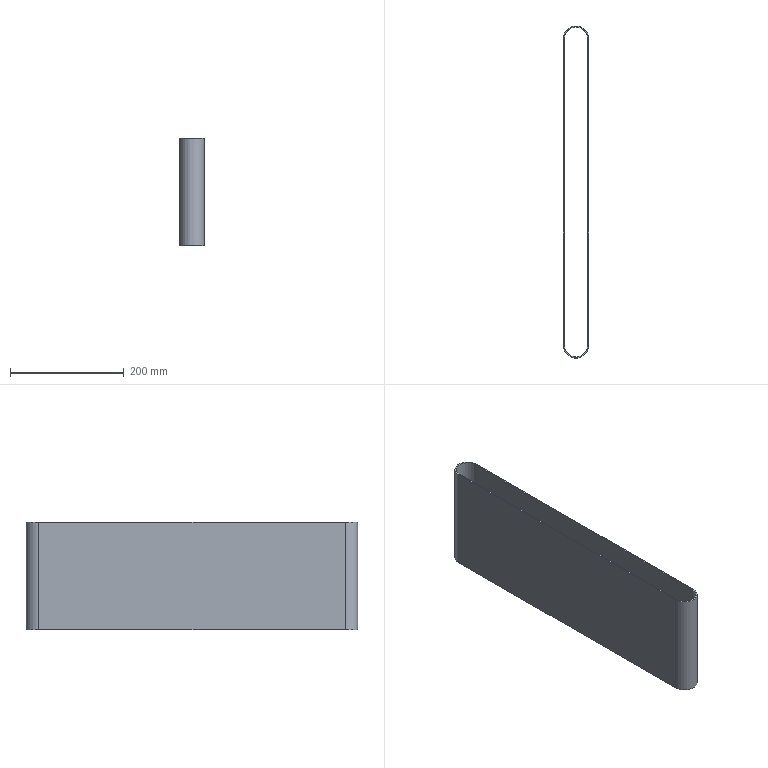Part | SolidWorks | features BeltProfileFeature 1, ExtruThin 1 | 1 solid | 10 faces | box 44.5 x 584.5 x 190 mm | volume 461137 mm3 | plane 6 | cylinder 4 | commonest cylinder face diameters 40.5 x2 44.5 x2
STEP:
#1=CARTESIAN_POINT('',(-22.25,0.,95.));
#2=VERTEX_POINT('',#1);
#3=CARTESIAN_POINT('',(22.25,0.,95.));
#4=VERTEX_POINT('',#3);
#5=CARTESIAN_POINT('',(0.,0.,95.));
#6=DIRECTION('',(0.,0.,1.));
#7=DIRECTION('',(-1.,0.,0.));
#8=AXIS2_PLACEMENT_3D('',#5,#6,#7);
#9=CIRCLE('',#8,22.25);
#10=EDGE_CURVE('',#2,#4,#9,.T.);
#11=ORIENTED_EDGE('',*,*,#10,.T.);
#12=CARTESIAN_POINT('',(22.25,540.,95.));
#13=VERTEX_POINT('',#12);
#14=CARTESIAN_POINT('',(22.25,0.,95.));
#15=DIRECTION('',(0.,1.,0.));
#16=VECTOR('',#15,1000.);
#17=LINE('',#14,#16);
#18=EDGE_CURVE('',#4,#13,#17,.T.);
#19=ORIENTED_EDGE('',*,*,#18,.T.);
#20=CARTESIAN_POINT('',(-22.25,540.,95.));
#21=VERTEX_POINT('',#20);
#22=CARTESIAN_POINT('',(0.,540.,95.));
#23=DIRECTION('',(0.,0.,1.));
#24=DIRECTION('',(-1.,0.,0.));
#25=AXIS2_PLACEMENT_3D('',#22,#23,#24);
#26=CIRCLE('',#25,22.25);
#27=EDGE_CURVE('',#13,#21,#26,.T.);
#28=ORIENTED_EDGE('',*,*,#27,.T.);
#29=CARTESIAN_POINT('',(-22.25,0.,95.));
#30=DIRECTION('',(0.,-1.,0.));
#31=VECTOR('',#30,1000.);
#32=LINE('',#29,#31);
#33=EDGE_CURVE('',#21,#2,#32,.T.);
#34=ORIENTED_EDGE('',*,*,#33,.T.);
#35=EDGE_LOOP('',(#11,#19,#28,#34));
#36=FACE_OUTER_BOUND('',#35,.T.);
#37=CARTESIAN_POINT('',(-20.25,0.,95.));
#38=VERTEX_POINT('',#37);
#39=CARTESIAN_POINT('',(20.25,0.,95.));
#40=VERTEX_POINT('',#39);
#41=CARTESIAN_POINT('',(0.,0.,95.));
#42=DIRECTION('',(0.,0.,1.));
#43=DIRECTION('',(-1.,0.,0.));
#44=AXIS2_PLACEMENT_3D('',#41,#42,#43);
#45=CIRCLE('',#44,20.25);
#46=EDGE_CURVE('',#38,#40,#45,.T.);
#47=ORIENTED_EDGE('',*,*,#46,.F.);
#48=CARTESIAN_POINT('',(-20.25,540.,95.));
#49=VERTEX_POINT('',#48);
#50=CARTESIAN_POINT('',(-20.25,0.,95.));
#51=DIRECTION('',(0.,-1.,0.));
#52=VECTOR('',#51,1000.);
#53=LINE('',#50,#52);
#54=EDGE_CURVE('',#49,#38,#53,.T.);
#55=ORIENTED_EDGE('',*,*,#54,.F.);
#56=CARTESIAN_POINT('',(20.25,540.,95.));
#57=VERTEX_POINT('',#56);
#58=CARTESIAN_POINT('',(0.,540.,95.));
#59=DIRECTION('',(0.,0.,1.));
#60=DIRECTION('',(-1.,0.,0.));
#61=AXIS2_PLACEMENT_3D('',#58,#59,#60);
#62=CIRCLE('',#61,20.25);
#63=EDGE_CURVE('',#57,#49,#62,.T.);
#64=ORIENTED_EDGE('',*,*,#63,.F.);
#65=CARTESIAN_POINT('',(20.25,540.,95.));
#66=DIRECTION('',(0.,1.,0.));
#67=VECTOR('',#66,1000.);
#68=LINE('',#65,#67);
#69=EDGE_CURVE('',#40,#57,#68,.T.);
#70=ORIENTED_EDGE('',*,*,#69,.F.);
#71=EDGE_LOOP('',(#47,#55,#64,#70));
#72=FACE_BOUND('',#71,.T.);
#73=CARTESIAN_POINT('',(0.,0.,95.));
#74=DIRECTION('',(0.,0.,-1.));
#75=DIRECTION('',(-1.,0.,0.));
#76=AXIS2_PLACEMENT_3D('',#73,#74,#75);
#77=PLANE('',#76);
#78=ADVANCED_FACE('',(#36,#72),#77,.F.);
#79=CARTESIAN_POINT('',(-22.25,0.,-95.));
#80=VERTEX_POINT('',#79);
#81=CARTESIAN_POINT('',(22.25,0.,-95.));
#82=VERTEX_POINT('',#81);
#83=CARTESIAN_POINT('',(0.,0.,-95.));
#84=DIRECTION('',(0.,0.,1.));
#85=DIRECTION('',(-1.,0.,0.));
#86=AXIS2_PLACEMENT_3D('',#83,#84,#85);
#87=CIRCLE('',#86,22.25);
#88=EDGE_CURVE('',#80,#82,#87,.T.);
#89=ORIENTED_EDGE('',*,*,#88,.F.);
#90=CARTESIAN_POINT('',(-22.25,540.,-95.));
#91=VERTEX_POINT('',#90);
#92=CARTESIAN_POINT('',(-22.25,0.,-95.));
#93=DIRECTION('',(0.,-1.,0.));
#94=VECTOR('',#93,1000.);
#95=LINE('',#92,#94);
#96=EDGE_CURVE('',#91,#80,#95,.T.);
#97=ORIENTED_EDGE('',*,*,#96,.F.);
#98=CARTESIAN_POINT('',(22.25,540.,-95.));
#99=VERTEX_POINT('',#98);
#100=CARTESIAN_POINT('',(0.,540.,-95.));
#101=DIRECTION('',(0.,0.,1.));
#102=DIRECTION('',(-1.,0.,0.));
#103=AXIS2_PLACEMENT_3D('',#100,#101,#102);
#104=CIRCLE('',#103,22.25);
#105=EDGE_CURVE('',#99,#91,#104,.T.);
#106=ORIENTED_EDGE('',*,*,#105,.F.);
#107=CARTESIAN_POINT('',(22.25,0.,-95.));
#108=DIRECTION('',(0.,1.,0.));
#109=VECTOR('',#108,1000.);
#110=LINE('',#107,#109);
#111=EDGE_CURVE('',#82,#99,#110,.T.);
#112=ORIENTED_EDGE('',*,*,#111,.F.);
#113=EDGE_LOOP('',(#89,#97,#106,#112));
#114=FACE_OUTER_BOUND('',#113,.T.);
#115=CARTESIAN_POINT('',(-20.25,540.,-95.));
#116=VERTEX_POINT('',#115);
#117=CARTESIAN_POINT('',(-20.25,0.,-95.));
#118=VERTEX_POINT('',#117);
#119=CARTESIAN_POINT('',(-20.25,0.,-95.));
#120=DIRECTION('',(0.,-1.,0.));
#121=VECTOR('',#120,1000.);
#122=LINE('',#119,#121);
#123=EDGE_CURVE('',#116,#118,#122,.T.);
#124=ORIENTED_EDGE('',*,*,#123,.T.);
#125=CARTESIAN_POINT('',(20.25,0.,-95.));
#126=VERTEX_POINT('',#125);
#127=CARTESIAN_POINT('',(0.,0.,-95.));
#128=DIRECTION('',(0.,0.,1.));
#129=DIRECTION('',(-1.,0.,0.));
#130=AXIS2_PLACEMENT_3D('',#127,#128,#129);
#131=CIRCLE('',#130,20.25);
#132=EDGE_CURVE('',#118,#126,#131,.T.);
#133=ORIENTED_EDGE('',*,*,#132,.T.);
#134=CARTESIAN_POINT('',(20.25,540.,-95.));
#135=VERTEX_POINT('',#134);
#136=CARTESIAN_POINT('',(20.25,540.,-95.));
#137=DIRECTION('',(0.,1.,0.));
#138=VECTOR('',#137,1000.);
#139=LINE('',#136,#138);
#140=EDGE_CURVE('',#126,#135,#139,.T.);
#141=ORIENTED_EDGE('',*,*,#140,.T.);
#142=CARTESIAN_POINT('',(0.,540.,-95.));
#143=DIRECTION('',(0.,0.,1.));
#144=DIRECTION('',(-1.,0.,0.));
#145=AXIS2_PLACEMENT_3D('',#142,#143,#144);
#146=CIRCLE('',#145,20.25);
#147=EDGE_CURVE('',#135,#116,#146,.T.);
#148=ORIENTED_EDGE('',*,*,#147,.T.);
#149=EDGE_LOOP('',(#124,#133,#141,#148));
#150=FACE_BOUND('',#149,.T.);
#151=CARTESIAN_POINT('',(0.,0.,-95.));
#152=DIRECTION('',(0.,0.,-1.));
#153=DIRECTION('',(-1.,0.,0.));
#154=AXIS2_PLACEMENT_3D('',#151,#152,#153);
#155=PLANE('',#154);
#156=ADVANCED_FACE('',(#114,#150),#155,.T.);
#157=ORIENTED_EDGE('',*,*,#88,.T.);
#158=CARTESIAN_POINT('',(22.25,0.,95.));
#159=DIRECTION('',(0.,0.,-1.));
#160=VECTOR('',#159,1000.);
#161=LINE('',#158,#160);
#162=EDGE_CURVE('',#4,#82,#161,.T.);
#163=ORIENTED_EDGE('',*,*,#162,.F.);
#164=ORIENTED_EDGE('',*,*,#10,.F.);
#165=CARTESIAN_POINT('',(-22.25,0.,95.));
#166=DIRECTION('',(0.,0.,-1.));
#167=VECTOR('',#166,1000.);
#168=LINE('',#165,#167);
#169=EDGE_CURVE('',#2,#80,#168,.T.);
#170=ORIENTED_EDGE('',*,*,#169,.T.);
#171=EDGE_LOOP('',(#157,#163,#164,#170));
#172=FACE_OUTER_BOUND('',#171,.T.);
#173=CARTESIAN_POINT('',(0.,0.,95.));
#174=DIRECTION('',(0.,0.,-1.));
#175=DIRECTION('',(-1.,0.,0.));
#176=AXIS2_PLACEMENT_3D('',#173,#174,#175);
#177=CYLINDRICAL_SURFACE('',#176,22.25);
#178=ADVANCED_FACE('',(#172),#177,.T.);
#179=ORIENTED_EDGE('',*,*,#111,.T.);
#180=CARTESIAN_POINT('',(22.25,540.,95.));
#181=DIRECTION('',(0.,0.,-1.));
#182=VECTOR('',#181,1000.);
#183=LINE('',#180,#182);
#184=EDGE_CURVE('',#13,#99,#183,.T.);
#185=ORIENTED_EDGE('',*,*,#184,.F.);
#186=ORIENTED_EDGE('',*,*,#18,.F.);
#187=ORIENTED_EDGE('',*,*,#162,.T.);
#188=EDGE_LOOP('',(#179,#185,#186,#187));
#189=FACE_OUTER_BOUND('',#188,.T.);
#190=CARTESIAN_POINT('',(22.25,0.,95.));
#191=DIRECTION('',(-1.,0.,0.));
#192=DIRECTION('',(0.,-1.,0.));
#193=AXIS2_PLACEMENT_3D('',#190,#191,#192);
#194=PLANE('',#193);
#195=ADVANCED_FACE('',(#189),#194,.F.);
#196=ORIENTED_EDGE('',*,*,#105,.T.);
#197=CARTESIAN_POINT('',(-22.25,540.,95.));
#198=DIRECTION('',(0.,0.,-1.));
#199=VECTOR('',#198,1000.);
#200=LINE('',#197,#199);
#201=EDGE_CURVE('',#21,#91,#200,.T.);
#202=ORIENTED_EDGE('',*,*,#201,.F.);
#203=ORIENTED_EDGE('',*,*,#27,.F.);
#204=ORIENTED_EDGE('',*,*,#184,.T.);
#205=EDGE_LOOP('',(#196,#202,#203,#204));
#206=FACE_OUTER_BOUND('',#205,.T.);
#207=CARTESIAN_POINT('',(0.,540.,95.));
#208=DIRECTION('',(0.,0.,-1.));
#209=DIRECTION('',(-1.,0.,0.));
#210=AXIS2_PLACEMENT_3D('',#207,#208,#209);
#211=CYLINDRICAL_SURFACE('',#210,22.25);
#212=ADVANCED_FACE('',(#206),#211,.T.);
#213=ORIENTED_EDGE('',*,*,#96,.T.);
#214=ORIENTED_EDGE('',*,*,#169,.F.);
#215=ORIENTED_EDGE('',*,*,#33,.F.);
#216=ORIENTED_EDGE('',*,*,#201,.T.);
#217=EDGE_LOOP('',(#213,#214,#215,#216));
#218=FACE_OUTER_BOUND('',#217,.T.);
#219=CARTESIAN_POINT('',(-22.25,0.,95.));
#220=DIRECTION('',(1.,0.,0.));
#221=DIRECTION('',(0.,1.,0.));
#222=AXIS2_PLACEMENT_3D('',#219,#220,#221);
#223=PLANE('',#222);
#224=ADVANCED_FACE('',(#218),#223,.F.);
#225=ORIENTED_EDGE('',*,*,#132,.F.);
#226=CARTESIAN_POINT('',(-20.25,0.,95.));
#227=DIRECTION('',(0.,0.,-1.));
#228=VECTOR('',#227,1000.);
#229=LINE('',#226,#228);
#230=EDGE_CURVE('',#38,#118,#229,.T.);
#231=ORIENTED_EDGE('',*,*,#230,.F.);
#232=ORIENTED_EDGE('',*,*,#46,.T.);
#233=CARTESIAN_POINT('',(20.25,0.,95.));
#234=DIRECTION('',(0.,0.,-1.));
#235=VECTOR('',#234,1000.);
#236=LINE('',#233,#235);
#237=EDGE_CURVE('',#40,#126,#236,.T.);
#238=ORIENTED_EDGE('',*,*,#237,.T.);
#239=EDGE_LOOP('',(#225,#231,#232,#238));
#240=FACE_OUTER_BOUND('',#239,.T.);
#241=CARTESIAN_POINT('',(0.,0.,95.));
#242=DIRECTION('',(0.,0.,-1.));
#243=DIRECTION('',(-1.,0.,0.));
#244=AXIS2_PLACEMENT_3D('',#241,#242,#243);
#245=CYLINDRICAL_SURFACE('',#244,20.25);
#246=ADVANCED_FACE('',(#240),#245,.F.);
#247=ORIENTED_EDGE('',*,*,#140,.F.);
#248=ORIENTED_EDGE('',*,*,#237,.F.);
#249=ORIENTED_EDGE('',*,*,#69,.T.);
#250=CARTESIAN_POINT('',(20.25,540.,95.));
#251=DIRECTION('',(0.,0.,-1.));
#252=VECTOR('',#251,1000.);
#253=LINE('',#250,#252);
#254=EDGE_CURVE('',#57,#135,#253,.T.);
#255=ORIENTED_EDGE('',*,*,#254,.T.);
#256=EDGE_LOOP('',(#247,#248,#249,#255));
#257=FACE_OUTER_BOUND('',#256,.T.);
#258=CARTESIAN_POINT('',(20.25,540.,95.));
#259=DIRECTION('',(-1.,0.,0.));
#260=DIRECTION('',(0.,-1.,0.));
#261=AXIS2_PLACEMENT_3D('',#258,#259,#260);
#262=PLANE('',#261);
#263=ADVANCED_FACE('',(#257),#262,.T.);
#264=ORIENTED_EDGE('',*,*,#147,.F.);
#265=ORIENTED_EDGE('',*,*,#254,.F.);
#266=ORIENTED_EDGE('',*,*,#63,.T.);
#267=CARTESIAN_POINT('',(-20.25,540.,95.));
#268=DIRECTION('',(0.,0.,-1.));
#269=VECTOR('',#268,1000.);
#270=LINE('',#267,#269);
#271=EDGE_CURVE('',#49,#116,#270,.T.);
#272=ORIENTED_EDGE('',*,*,#271,.T.);
#273=EDGE_LOOP('',(#264,#265,#266,#272));
#274=FACE_OUTER_BOUND('',#273,.T.);
#275=CARTESIAN_POINT('',(0.,540.,95.));
#276=DIRECTION('',(0.,0.,-1.));
#277=DIRECTION('',(-1.,0.,0.));
#278=AXIS2_PLACEMENT_3D('',#275,#276,#277);
#279=CYLINDRICAL_SURFACE('',#278,20.25);
#280=ADVANCED_FACE('',(#274),#279,.F.);
#281=ORIENTED_EDGE('',*,*,#123,.F.);
#282=ORIENTED_EDGE('',*,*,#271,.F.);
#283=ORIENTED_EDGE('',*,*,#54,.T.);
#284=ORIENTED_EDGE('',*,*,#230,.T.);
#285=EDGE_LOOP('',(#281,#282,#283,#284));
#286=FACE_OUTER_BOUND('',#285,.T.);
#287=CARTESIAN_POINT('',(-20.25,0.,95.));
#288=DIRECTION('',(1.,0.,0.));
#289=DIRECTION('',(0.,1.,0.));
#290=AXIS2_PLACEMENT_3D('',#287,#288,#289);
#291=PLANE('',#290);
#292=ADVANCED_FACE('',(#286),#291,.T.);
#293=CLOSED_SHELL('',(#78,#156,#178,#195,#212,#224,#246,#263,#280,#292));
#294=MANIFOLD_SOLID_BREP('',#293);
#295=CARTESIAN_POINT('',(0.,0.,0.));
#296=DIRECTION('',(0.,0.,1.));
#297=DIRECTION('',(1.,0.,0.));
#298=AXIS2_PLACEMENT_3D('',#295,#296,#297);
#299=(LENGTH_UNIT()NAMED_UNIT(*)SI_UNIT(.MILLI.,.METRE.));
#300=UNCERTAINTY_MEASURE_WITH_UNIT(LENGTH_MEASURE(0.00001),#299,'','');
#301=(NAMED_UNIT(*)PLANE_ANGLE_UNIT()SI_UNIT($,.RADIAN.));
#302=(NAMED_UNIT(*)SI_UNIT($,.STERADIAN.)SOLID_ANGLE_UNIT());
#303=(GEOMETRIC_REPRESENTATION_CONTEXT(3)GLOBAL_UNCERTAINTY_ASSIGNED_CONTEXT((#300))GLOBAL_UNIT_ASSIGNED_CONTEXT((#299,#301,#302))REPRESENTATION_CONTEXT('',''));
#304=ADVANCED_BREP_SHAPE_REPRESENTATION('',(#294,#298),#303);